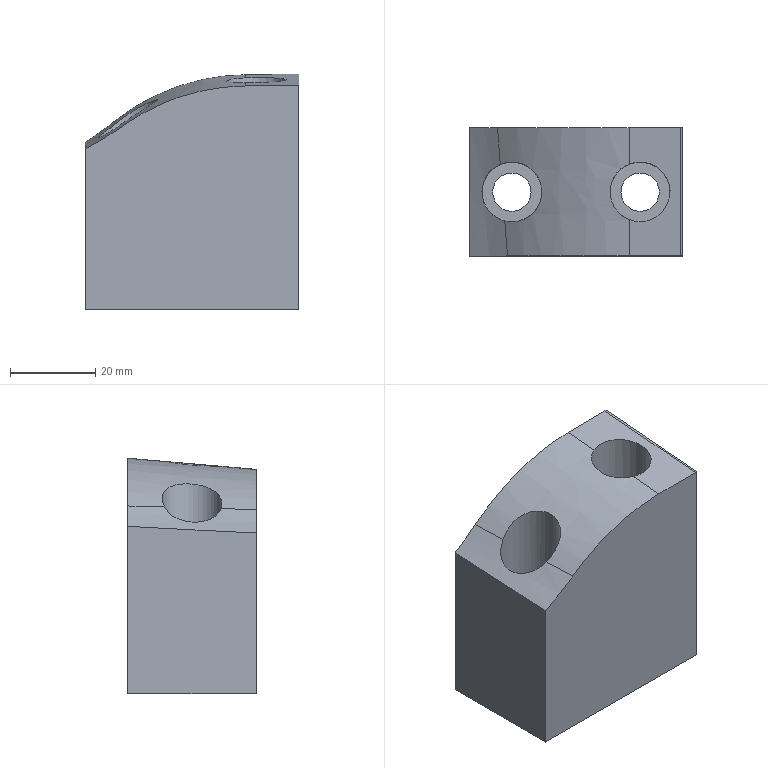Part | NX | features solid 2 | 1 solid | 15 faces | box 50 x 30 x 55.131 mm | volume 61249 mm3 | plane 7 | cylinder 4 | spline 4 | commonest cylinder face diameters 9 x2 14 x2
STEP:
#1=CARTESIAN_POINT('',(822.5,150.,1.131));
#2=VERTEX_POINT('',#1);
#3=CARTESIAN_POINT('',(822.5,150.,-54.));
#4=VERTEX_POINT('',#3);
#5=CARTESIAN_POINT('',(822.5,150.,41.));
#6=DIRECTION('',(0.,0.,-1.));
#7=VECTOR('',#6,1000.);
#8=LINE('',#5,#7);
#9=EDGE_CURVE('',#2,#4,#8,.T.);
#10=ORIENTED_EDGE('',*,*,#9,.F.);
#11=CARTESIAN_POINT('',(822.5,120.,-1.493));
#12=VERTEX_POINT('',#11);
#13=CARTESIAN_POINT('',(822.5,153.462,1.434));
#14=DIRECTION('',(0.,-0.9962,-0.08716));
#15=VECTOR('',#14,1000.);
#16=LINE('',#13,#15);
#17=EDGE_CURVE('',#2,#12,#16,.T.);
#18=ORIENTED_EDGE('',*,*,#17,.T.);
#19=CARTESIAN_POINT('',(822.5,120.,-54.));
#20=VERTEX_POINT('',#19);
#21=CARTESIAN_POINT('',(822.5,120.,41.));
#22=DIRECTION('',(0.,0.,-1.));
#23=VECTOR('',#22,1000.);
#24=LINE('',#21,#23);
#25=EDGE_CURVE('',#12,#20,#24,.T.);
#26=ORIENTED_EDGE('',*,*,#25,.T.);
#27=CARTESIAN_POINT('',(822.5,150.,-54.));
#28=DIRECTION('',(0.,1.,0.));
#29=VECTOR('',#28,1000.);
#30=LINE('',#27,#29);
#31=EDGE_CURVE('',#4,#20,#30,.F.);
#32=ORIENTED_EDGE('',*,*,#31,.F.);
#33=EDGE_LOOP('',(#10,#18,#26,#32));
#34=FACE_BOUND('',#33,.T.);
#35=CARTESIAN_POINT('',(822.5,150.,41.));
#36=DIRECTION('',(1.,0.,0.));
#37=DIRECTION('',(0.,0.,-1.));
#38=AXIS2_PLACEMENT_3D('',#35,#36,#37);
#39=PLANE('',#38);
#40=ADVANCED_FACE('',(#34),#39,.T.);
#41=CARTESIAN_POINT('',(805.5,135.,-44.));
#42=VERTEX_POINT('',#41);
#43=CARTESIAN_POINT('',(812.5,135.,-44.));
#44=DIRECTION('',(0.,0.,-1.));
#45=DIRECTION('',(-1.,0.,0.));
#46=AXIS2_PLACEMENT_3D('',#43,#44,#45);
#47=CIRCLE('',#46,7.);
#48=EDGE_CURVE('',#42,#42,#47,.T.);
#49=ORIENTED_EDGE('',*,*,#48,.T.);
#50=EDGE_LOOP('',(#49));
#51=FACE_BOUND('',#50,.T.);
#52=CARTESIAN_POINT('',(809.928,128.49,-0.8829));
#53=VERTEX_POINT('',#52);
#54=CARTESIAN_POINT('',(809.924,141.509,0.2561));
#55=VERTEX_POINT('',#54);
#56=CARTESIAN_POINT('',(809.929,128.489,-0.8829));
#57=CARTESIAN_POINT('',(808.616,129.008,-0.8514));
#58=CARTESIAN_POINT('',(806.357,130.826,-0.826));
#59=CARTESIAN_POINT('',(805.067,135.021,-0.6039));
#60=CARTESIAN_POINT('',(806.373,139.185,-0.09322));
#61=CARTESIAN_POINT('',(808.613,140.99,0.1969));
#62=CARTESIAN_POINT('',(809.924,141.509,0.2561));
#63=B_SPLINE_CURVE_WITH_KNOTS('',3,(#56,#57,#58,#59,#60,#61,#62),.UNSPECIFIED.,.F.,.F.,(4,1,1,1,4),(0.,0.004174,0.008348,0.01252,0.0167),.UNSPECIFIED.);
#64=EDGE_CURVE('',#53,#55,#63,.T.);
#65=ORIENTED_EDGE('',*,*,#64,.F.);
#66=CARTESIAN_POINT('',(809.923,141.509,0.2561));
#67=CARTESIAN_POINT('',(812.027,142.341,0.351));
#68=CARTESIAN_POINT('',(817.119,141.772,0.3547));
#69=CARTESIAN_POINT('',(820.693,134.994,-0.2007));
#70=CARTESIAN_POINT('',(817.109,128.237,-0.8296));
#71=CARTESIAN_POINT('',(812.055,127.649,-0.9341));
#72=CARTESIAN_POINT('',(809.927,128.49,-0.8829));
#73=B_SPLINE_CURVE_WITH_KNOTS('',3,(#66,#67,#68,#69,#70,#71,#72),.UNSPECIFIED.,.F.,.F.,(4,1,1,1,4),(0.008341,0.01514,0.02193,0.02872,0.03552),.UNSPECIFIED.);
#74=EDGE_CURVE('',#55,#53,#73,.T.);
#75=ORIENTED_EDGE('',*,*,#74,.F.);
#76=EDGE_LOOP('',(#65,#75));
#77=FACE_BOUND('',#76,.T.);
#78=CARTESIAN_POINT('',(812.5,135.,41.));
#79=DIRECTION('',(0.,0.,-1.));
#80=DIRECTION('',(-1.,0.,0.));
#81=AXIS2_PLACEMENT_3D('',#78,#79,#80);
#82=CYLINDRICAL_SURFACE('',#81,7.);
#83=ADVANCED_FACE('',(#51,#77),#82,.F.);
#84=CARTESIAN_POINT('',(775.5,135.,-44.));
#85=VERTEX_POINT('',#84);
#86=CARTESIAN_POINT('',(782.5,135.,-44.));
#87=DIRECTION('',(0.,0.,-1.));
#88=DIRECTION('',(-1.,0.,0.));
#89=AXIS2_PLACEMENT_3D('',#86,#87,#88);
#90=CIRCLE('',#89,7.);
#91=EDGE_CURVE('',#85,#85,#90,.T.);
#92=ORIENTED_EDGE('',*,*,#91,.T.);
#93=EDGE_LOOP('',(#92));
#94=FACE_BOUND('',#93,.T.);
#95=CARTESIAN_POINT('',(779.784,141.451,-10.294));
#96=VERTEX_POINT('',#95);
#97=CARTESIAN_POINT('',(780.817,128.205,-10.671));
#98=VERTEX_POINT('',#97);
#99=CARTESIAN_POINT('',(779.784,141.451,-10.294));
#100=CARTESIAN_POINT('',(780.681,141.829,-9.561));
#101=CARTESIAN_POINT('',(782.626,142.218,-8.111));
#102=CARTESIAN_POINT('',(785.785,141.482,-6.226));
#103=CARTESIAN_POINT('',(788.514,139.168,-5.014));
#104=CARTESIAN_POINT('',(789.811,135.579,-4.738));
#105=CARTESIAN_POINT('',(789.108,131.88,-5.377));
#106=CARTESIAN_POINT('',(786.834,129.171,-6.736));
#107=CARTESIAN_POINT('',(783.84,127.898,-8.579));
#108=CARTESIAN_POINT('',(781.792,127.964,-9.973));
#109=CARTESIAN_POINT('',(780.818,128.205,-10.671));
#110=B_SPLINE_CURVE_WITH_KNOTS('',3,(#99,#100,#101,#102,#103,#104,#105,#106,#107,#108,#109),.UNSPECIFIED.,.F.,.F.,(4,1,1,1,1,1,1,1,4),(0.009346,0.01299,0.01663,0.02027,0.02391,0.02755,0.03119,0.03483,0.03847),.UNSPECIFIED.);
#111=EDGE_CURVE('',#96,#98,#110,.T.);
#112=ORIENTED_EDGE('',*,*,#111,.F.);
#113=CARTESIAN_POINT('',(779.784,141.451,-10.294));
#114=CARTESIAN_POINT('',(778.607,140.956,-11.254));
#115=CARTESIAN_POINT('',(776.389,139.3,-12.978));
#116=CARTESIAN_POINT('',(774.925,134.527,-14.202));
#117=CARTESIAN_POINT('',(776.996,129.903,-13.211));
#118=CARTESIAN_POINT('',(779.54,128.522,-11.587));
#119=CARTESIAN_POINT('',(780.816,128.205,-10.672));
#120=B_SPLINE_CURVE_WITH_KNOTS('',3,(#113,#114,#115,#116,#117,#118,#119),.UNSPECIFIED.,.F.,.F.,(4,1,1,1,4),(0.,0.004707,0.009414,0.01412,0.01883),.UNSPECIFIED.);
#121=EDGE_CURVE('',#96,#98,#120,.T.);
#122=ORIENTED_EDGE('',*,*,#121,.T.);
#123=EDGE_LOOP('',(#112,#122));
#124=FACE_BOUND('',#123,.T.);
#125=CARTESIAN_POINT('',(782.5,135.,41.));
#126=DIRECTION('',(0.,0.,-1.));
#127=DIRECTION('',(-1.,0.,0.));
#128=AXIS2_PLACEMENT_3D('',#125,#126,#127);
#129=CYLINDRICAL_SURFACE('',#128,7.);
#130=ADVANCED_FACE('',(#94,#124),#129,.F.);
#131=CARTESIAN_POINT('',(779.144,150.,-10.05));
#132=VERTEX_POINT('',#131);
#133=CARTESIAN_POINT('',(772.5,150.,-14.808));
#134=VERTEX_POINT('',#133);
#135=CARTESIAN_POINT('',(779.144,150.,-10.05));
#136=CARTESIAN_POINT('',(777.019,150.,-11.762));
#137=CARTESIAN_POINT('',(774.805,150.,-13.348));
#138=CARTESIAN_POINT('',(772.5,150.,-14.808));
#139=B_SPLINE_CURVE_WITH_KNOTS('',3,(#135,#136,#137,#138),.UNSPECIFIED.,.F.,.F.,(4,4),(0.,0.008172),.UNSPECIFIED.);
#140=EDGE_CURVE('',#132,#134,#139,.T.);
#141=ORIENTED_EDGE('',*,*,#140,.F.);
#142=CARTESIAN_POINT('',(809.92,150.,0.9989));
#143=VERTEX_POINT('',#142);
#144=CARTESIAN_POINT('',(779.144,150.,-10.05));
#145=CARTESIAN_POINT('',(781.291,150.,-8.319));
#146=CARTESIAN_POINT('',(785.926,150.,-5.181));
#147=CARTESIAN_POINT('',(796.008,150.,-0.576));
#148=CARTESIAN_POINT('',(804.326,150.,0.9401));
#149=CARTESIAN_POINT('',(809.921,150.,0.9989));
#150=B_SPLINE_CURVE_WITH_KNOTS('',3,(#144,#145,#146,#147,#148,#149),.UNSPECIFIED.,.F.,.F.,(4,1,1,4),(0.009236,0.01751,0.02578,0.04233),.UNSPECIFIED.);
#151=EDGE_CURVE('',#132,#143,#150,.T.);
#152=ORIENTED_EDGE('',*,*,#151,.T.);
#153=CARTESIAN_POINT('',(821.971,150.,1.126));
#154=VERTEX_POINT('',#153);
#155=CARTESIAN_POINT('',(809.92,150.,0.9989));
#156=CARTESIAN_POINT('',(813.937,150.,1.041));
#157=CARTESIAN_POINT('',(817.954,150.,1.083));
#158=CARTESIAN_POINT('',(821.971,150.,1.126));
#159=B_SPLINE_CURVE_WITH_KNOTS('',3,(#155,#156,#157,#158),.UNSPECIFIED.,.F.,.F.,(4,4),(0.007434,0.01949),.UNSPECIFIED.);
#160=EDGE_CURVE('',#143,#154,#159,.T.);
#161=ORIENTED_EDGE('',*,*,#160,.T.);
#162=CARTESIAN_POINT('',(822.919,150.,1.136));
#163=DIRECTION('',(-0.9999,0.,-0.01051));
#164=VECTOR('',#163,1000.);
#165=LINE('',#162,#164);
#166=EDGE_CURVE('',#154,#2,#165,.F.);
#167=ORIENTED_EDGE('',*,*,#166,.T.);
#168=ORIENTED_EDGE('',*,*,#9,.T.);
#169=CARTESIAN_POINT('',(772.5,150.,-54.));
#170=VERTEX_POINT('',#169);
#171=CARTESIAN_POINT('',(822.5,150.,-54.));
#172=DIRECTION('',(-1.,0.,0.));
#173=VECTOR('',#172,1000.);
#174=LINE('',#171,#173);
#175=EDGE_CURVE('',#4,#170,#174,.T.);
#176=ORIENTED_EDGE('',*,*,#175,.T.);
#177=CARTESIAN_POINT('',(772.5,150.,41.));
#178=DIRECTION('',(0.,0.,-1.));
#179=VECTOR('',#178,1000.);
#180=LINE('',#177,#179);
#181=EDGE_CURVE('',#134,#170,#180,.T.);
#182=ORIENTED_EDGE('',*,*,#181,.F.);
#183=EDGE_LOOP('',(#141,#152,#161,#167,#168,#176,#182));
#184=FACE_BOUND('',#183,.T.);
#185=CARTESIAN_POINT('',(822.5,150.,41.));
#186=DIRECTION('',(0.,-1.,0.));
#187=DIRECTION('',(0.,0.,-1.));
#188=AXIS2_PLACEMENT_3D('',#185,#186,#187);
#189=PLANE('',#188);
#190=ADVANCED_FACE('',(#184),#189,.F.);
#191=CARTESIAN_POINT('',(787.,135.,-54.));
#192=VERTEX_POINT('',#191);
#193=CARTESIAN_POINT('',(782.5,135.,-54.));
#194=DIRECTION('',(0.,0.,1.));
#195=DIRECTION('',(1.,0.,0.));
#196=AXIS2_PLACEMENT_3D('',#193,#194,#195);
#197=CIRCLE('',#196,4.5);
#198=EDGE_CURVE('',#192,#192,#197,.F.);
#199=ORIENTED_EDGE('',*,*,#198,.F.);
#200=EDGE_LOOP('',(#199));
#201=FACE_BOUND('',#200,.T.);
#202=CARTESIAN_POINT('',(817.,135.,-54.));
#203=VERTEX_POINT('',#202);
#204=CARTESIAN_POINT('',(812.5,135.,-54.));
#205=DIRECTION('',(0.,0.,1.));
#206=DIRECTION('',(1.,0.,0.));
#207=AXIS2_PLACEMENT_3D('',#204,#205,#206);
#208=CIRCLE('',#207,4.5);
#209=EDGE_CURVE('',#203,#203,#208,.F.);
#210=ORIENTED_EDGE('',*,*,#209,.F.);
#211=EDGE_LOOP('',(#210));
#212=FACE_BOUND('',#211,.T.);
#213=ORIENTED_EDGE('',*,*,#175,.F.);
#214=ORIENTED_EDGE('',*,*,#31,.T.);
#215=CARTESIAN_POINT('',(772.5,120.,-54.));
#216=VERTEX_POINT('',#215);
#217=CARTESIAN_POINT('',(822.5,120.,-54.));
#218=DIRECTION('',(1.,0.,0.));
#219=VECTOR('',#218,1000.);
#220=LINE('',#217,#219);
#221=EDGE_CURVE('',#20,#216,#220,.F.);
#222=ORIENTED_EDGE('',*,*,#221,.T.);
#223=CARTESIAN_POINT('',(772.5,150.,-54.));
#224=DIRECTION('',(0.,1.,0.));
#225=VECTOR('',#224,1000.);
#226=LINE('',#223,#225);
#227=EDGE_CURVE('',#170,#216,#226,.F.);
#228=ORIENTED_EDGE('',*,*,#227,.F.);
#229=EDGE_LOOP('',(#213,#214,#222,#228));
#230=FACE_BOUND('',#229,.T.);
#231=CARTESIAN_POINT('',(822.5,150.,-54.));
#232=DIRECTION('',(0.,0.,1.));
#233=DIRECTION('',(0.,-1.,0.));
#234=AXIS2_PLACEMENT_3D('',#231,#232,#233);
#235=PLANE('',#234);
#236=ADVANCED_FACE('',(#201,#212,#230),#235,.F.);
#237=CARTESIAN_POINT('',(772.5,120.,-16.381));
#238=VERTEX_POINT('',#237);
#239=CARTESIAN_POINT('',(781.483,120.,-10.907));
#240=VERTEX_POINT('',#239);
#241=CARTESIAN_POINT('',(772.5,120.,-16.381));
#242=CARTESIAN_POINT('',(775.626,120.,-14.774));
#243=CARTESIAN_POINT('',(778.62,120.,-12.95));
#244=CARTESIAN_POINT('',(781.481,120.,-10.908));
#245=B_SPLINE_CURVE_WITH_KNOTS('',3,(#241,#242,#243,#244),.UNSPECIFIED.,.F.,.F.,(4,4),(0.,0.01052),.UNSPECIFIED.);
#246=EDGE_CURVE('',#238,#240,#245,.T.);
#247=ORIENTED_EDGE('',*,*,#246,.F.);
#248=CARTESIAN_POINT('',(772.5,120.,41.));
#249=DIRECTION('',(0.,0.,-1.));
#250=VECTOR('',#249,1000.);
#251=LINE('',#248,#250);
#252=EDGE_CURVE('',#238,#216,#251,.T.);
#253=ORIENTED_EDGE('',*,*,#252,.T.);
#254=ORIENTED_EDGE('',*,*,#221,.F.);
#255=ORIENTED_EDGE('',*,*,#25,.F.);
#256=CARTESIAN_POINT('',(821.971,120.,-1.499));
#257=VERTEX_POINT('',#256);
#258=CARTESIAN_POINT('',(822.947,120.,-1.489));
#259=DIRECTION('',(-0.9999,0.,-0.01051));
#260=VECTOR('',#259,1000.);
#261=LINE('',#258,#260);
#262=EDGE_CURVE('',#12,#257,#261,.T.);
#263=ORIENTED_EDGE('',*,*,#262,.T.);
#264=CARTESIAN_POINT('',(809.929,120.,-1.626));
#265=VERTEX_POINT('',#264);
#266=CARTESIAN_POINT('',(821.971,120.,-1.499));
#267=CARTESIAN_POINT('',(817.957,120.,-1.541));
#268=CARTESIAN_POINT('',(813.943,120.,-1.583));
#269=CARTESIAN_POINT('',(809.929,120.,-1.626));
#270=B_SPLINE_CURVE_WITH_KNOTS('',3,(#266,#267,#268,#269),.UNSPECIFIED.,.F.,.F.,(4,4),(0.,0.01204),.UNSPECIFIED.);
#271=EDGE_CURVE('',#257,#265,#270,.T.);
#272=ORIENTED_EDGE('',*,*,#271,.T.);
#273=CARTESIAN_POINT('',(809.93,120.,-1.626));
#274=CARTESIAN_POINT('',(804.815,120.,-1.679));
#275=CARTESIAN_POINT('',(797.323,120.,-2.914));
#276=CARTESIAN_POINT('',(787.852,120.,-6.826));
#277=CARTESIAN_POINT('',(783.548,120.,-9.433));
#278=CARTESIAN_POINT('',(781.484,120.,-10.906));
#279=B_SPLINE_CURVE_WITH_KNOTS('',3,(#273,#274,#275,#276,#277,#278),.UNSPECIFIED.,.F.,.F.,(4,1,1,4),(0.,0.01513,0.0227,0.03026),.UNSPECIFIED.);
#280=EDGE_CURVE('',#265,#240,#279,.T.);
#281=ORIENTED_EDGE('',*,*,#280,.T.);
#282=EDGE_LOOP('',(#247,#253,#254,#255,#263,#272,#281));
#283=FACE_BOUND('',#282,.T.);
#284=CARTESIAN_POINT('',(822.5,120.,41.));
#285=DIRECTION('',(0.,-1.,0.));
#286=DIRECTION('',(0.,0.,-1.));
#287=AXIS2_PLACEMENT_3D('',#284,#285,#286);
#288=PLANE('',#287);
#289=ADVANCED_FACE('',(#283),#288,.T.);
#290=ORIENTED_EDGE('',*,*,#252,.F.);
#291=CARTESIAN_POINT('',(772.5,120.,-16.381));
#292=CARTESIAN_POINT('',(772.5,130.003,-15.905));
#293=CARTESIAN_POINT('',(772.5,140.002,-15.38));
#294=CARTESIAN_POINT('',(772.5,150.,-14.808));
#295=B_SPLINE_CURVE_WITH_KNOTS('',3,(#291,#292,#293,#294),.UNSPECIFIED.,.F.,.F.,(4,4),(0.,0.03004),.UNSPECIFIED.);
#296=EDGE_CURVE('',#238,#134,#295,.T.);
#297=ORIENTED_EDGE('',*,*,#296,.T.);
#298=ORIENTED_EDGE('',*,*,#181,.T.);
#299=ORIENTED_EDGE('',*,*,#227,.T.);
#300=EDGE_LOOP('',(#290,#297,#298,#299));
#301=FACE_BOUND('',#300,.T.);
#302=CARTESIAN_POINT('',(772.5,150.,41.));
#303=DIRECTION('',(1.,0.,0.));
#304=DIRECTION('',(0.,0.,-1.));
#305=AXIS2_PLACEMENT_3D('',#302,#303,#304);
#306=PLANE('',#305);
#307=ADVANCED_FACE('',(#301),#306,.F.);
#308=ORIENTED_EDGE('',*,*,#209,.T.);
#309=EDGE_LOOP('',(#308));
#310=FACE_BOUND('',#309,.T.);
#311=CARTESIAN_POINT('',(808.,135.,-44.));
#312=VERTEX_POINT('',#311);
#313=CARTESIAN_POINT('',(812.5,135.,-44.));
#314=DIRECTION('',(0.,0.,-1.));
#315=DIRECTION('',(-1.,0.,0.));
#316=AXIS2_PLACEMENT_3D('',#313,#314,#315);
#317=CIRCLE('',#316,4.5);
#318=EDGE_CURVE('',#312,#312,#317,.T.);
#319=ORIENTED_EDGE('',*,*,#318,.F.);
#320=EDGE_LOOP('',(#319));
#321=FACE_BOUND('',#320,.T.);
#322=CARTESIAN_POINT('',(812.5,135.,-109.));
#323=DIRECTION('',(0.,0.,-1.));
#324=DIRECTION('',(-1.,0.,0.));
#325=AXIS2_PLACEMENT_3D('',#322,#323,#324);
#326=CYLINDRICAL_SURFACE('',#325,4.5);
#327=ADVANCED_FACE('',(#310,#321),#326,.F.);
#328=ORIENTED_EDGE('',*,*,#318,.T.);
#329=EDGE_LOOP('',(#328));
#330=FACE_BOUND('',#329,.T.);
#331=ORIENTED_EDGE('',*,*,#48,.F.);
#332=EDGE_LOOP('',(#331));
#333=FACE_BOUND('',#332,.T.);
#334=CARTESIAN_POINT('',(812.5,135.,-44.));
#335=DIRECTION('',(0.,0.,-1.));
#336=DIRECTION('',(-1.,0.,0.));
#337=AXIS2_PLACEMENT_3D('',#334,#335,#336);
#338=PLANE('',#337);
#339=ADVANCED_FACE('',(#330,#333),#338,.F.);
#340=ORIENTED_EDGE('',*,*,#198,.T.);
#341=EDGE_LOOP('',(#340));
#342=FACE_BOUND('',#341,.T.);
#343=CARTESIAN_POINT('',(778.,135.,-44.));
#344=VERTEX_POINT('',#343);
#345=CARTESIAN_POINT('',(782.5,135.,-44.));
#346=DIRECTION('',(0.,0.,-1.));
#347=DIRECTION('',(-1.,0.,0.));
#348=AXIS2_PLACEMENT_3D('',#345,#346,#347);
#349=CIRCLE('',#348,4.5);
#350=EDGE_CURVE('',#344,#344,#349,.T.);
#351=ORIENTED_EDGE('',*,*,#350,.F.);
#352=EDGE_LOOP('',(#351));
#353=FACE_BOUND('',#352,.T.);
#354=CARTESIAN_POINT('',(782.5,135.,-109.));
#355=DIRECTION('',(0.,0.,-1.));
#356=DIRECTION('',(-1.,0.,0.));
#357=AXIS2_PLACEMENT_3D('',#354,#355,#356);
#358=CYLINDRICAL_SURFACE('',#357,4.5);
#359=ADVANCED_FACE('',(#342,#353),#358,.F.);
#360=ORIENTED_EDGE('',*,*,#350,.T.);
#361=EDGE_LOOP('',(#360));
#362=FACE_BOUND('',#361,.T.);
#363=ORIENTED_EDGE('',*,*,#91,.F.);
#364=EDGE_LOOP('',(#363));
#365=FACE_BOUND('',#364,.T.);
#366=CARTESIAN_POINT('',(782.5,135.,-44.));
#367=DIRECTION('',(0.,0.,-1.));
#368=DIRECTION('',(-1.,0.,0.));
#369=AXIS2_PLACEMENT_3D('',#366,#367,#368);
#370=PLANE('',#369);
#371=ADVANCED_FACE('',(#362,#365),#370,.F.);
#372=ORIENTED_EDGE('',*,*,#160,.F.);
#373=CARTESIAN_POINT('',(809.923,141.509,0.2561));
#374=CARTESIAN_POINT('',(809.922,144.249,0.4958));
#375=CARTESIAN_POINT('',(809.921,147.08,0.7434));
#376=CARTESIAN_POINT('',(809.92,150.,0.9989));
#377=B_SPLINE_CURVE_WITH_KNOTS('',3,(#373,#374,#375,#376),.UNSPECIFIED.,.F.,.F.,(4,4),(0.8378,0.8517),.UNSPECIFIED.);
#378=EDGE_CURVE('',#55,#143,#377,.T.);
#379=ORIENTED_EDGE('',*,*,#378,.F.);
#380=ORIENTED_EDGE('',*,*,#74,.T.);
#381=CARTESIAN_POINT('',(809.929,120.,-1.626));
#382=CARTESIAN_POINT('',(809.929,122.697,-1.39));
#383=CARTESIAN_POINT('',(809.928,125.527,-1.142));
#384=CARTESIAN_POINT('',(809.927,128.49,-0.8829));
#385=B_SPLINE_CURVE_WITH_KNOTS('',3,(#381,#382,#383,#384),.UNSPECIFIED.,.F.,.F.,(4,4),(0.7976,0.8145),.UNSPECIFIED.);
#386=EDGE_CURVE('',#265,#53,#385,.T.);
#387=ORIENTED_EDGE('',*,*,#386,.F.);
#388=ORIENTED_EDGE('',*,*,#271,.F.);
#389=CARTESIAN_POINT('',(821.971,120.,-1.499));
#390=CARTESIAN_POINT('',(821.971,130.,-0.6242));
#391=CARTESIAN_POINT('',(821.971,140.,0.2507));
#392=CARTESIAN_POINT('',(821.971,150.,1.126));
#393=B_SPLINE_CURVE_WITH_KNOTS('',3,(#389,#390,#391,#392),.UNSPECIFIED.,.F.,.F.,(4,4),(0.3207,0.505),.UNSPECIFIED.);
#394=EDGE_CURVE('',#154,#257,#393,.F.);
#395=ORIENTED_EDGE('',*,*,#394,.F.);
#396=EDGE_LOOP('',(#372,#379,#380,#387,#388,#395));
#397=FACE_BOUND('',#396,.T.);
#398=CARTESIAN_POINT('',(809.848,119.82,-1.642));
#399=CARTESIAN_POINT('',(809.848,150.191,1.015));
#400=CARTESIAN_POINT('',(821.971,119.809,-1.516));
#401=CARTESIAN_POINT('',(821.971,150.18,1.141));
#402=B_SPLINE_SURFACE_WITH_KNOTS('',1,1,((#398,#399),(#400,#401)),.PLANE_SURF.,.F.,.F.,.F.,(2,2),(2,2),(0.8696,1.),(0.8254,0.8716),.PIECEWISE_BEZIER_KNOTS.);
#403=ADVANCED_FACE('',(#397),#402,.T.);
#404=ORIENTED_EDGE('',*,*,#151,.F.);
#405=CARTESIAN_POINT('',(779.144,150.,-10.05));
#406=CARTESIAN_POINT('',(779.249,148.57,-10.091));
#407=CARTESIAN_POINT('',(779.409,146.415,-10.152));
#408=CARTESIAN_POINT('',(779.624,143.552,-10.234));
#409=CARTESIAN_POINT('',(779.735,142.086,-10.276));
#410=CARTESIAN_POINT('',(779.784,141.451,-10.294));
#411=B_SPLINE_CURVE_WITH_KNOTS('',3,(#405,#406,#407,#408,#409,#410),.UNSPECIFIED.,.F.,.F.,(4,1,1,4),(0.2278,0.2397,0.2456,0.2516),.UNSPECIFIED.);
#412=EDGE_CURVE('',#132,#96,#411,.T.);
#413=ORIENTED_EDGE('',*,*,#412,.T.);
#414=ORIENTED_EDGE('',*,*,#111,.T.);
#415=CARTESIAN_POINT('',(780.818,128.205,-10.671));
#416=CARTESIAN_POINT('',(781.035,125.499,-10.748));
#417=CARTESIAN_POINT('',(781.257,122.764,-10.826));
#418=CARTESIAN_POINT('',(781.484,120.,-10.906));
#419=B_SPLINE_CURVE_WITH_KNOTS('',3,(#415,#416,#417,#418),.UNSPECIFIED.,.F.,.F.,(4,4),(0.2921,0.3165),.UNSPECIFIED.);
#420=EDGE_CURVE('',#98,#240,#419,.T.);
#421=ORIENTED_EDGE('',*,*,#420,.T.);
#422=ORIENTED_EDGE('',*,*,#280,.F.);
#423=ORIENTED_EDGE('',*,*,#386,.T.);
#424=ORIENTED_EDGE('',*,*,#64,.T.);
#425=ORIENTED_EDGE('',*,*,#378,.T.);
#426=EDGE_LOOP('',(#404,#413,#414,#421,#422,#423,#424,#425));
#427=FACE_BOUND('',#426,.T.);
#428=CARTESIAN_POINT('',(809.93,119.012,-1.712));
#429=CARTESIAN_POINT('',(792.527,119.027,-1.894));
#430=CARTESIAN_POINT('',(778.998,119.979,-12.802));
#431=CARTESIAN_POINT('',(809.929,129.403,-0.803));
#432=CARTESIAN_POINT('',(792.526,129.414,-0.985));
#433=CARTESIAN_POINT('',(778.997,130.364,-11.893));
#434=CARTESIAN_POINT('',(809.925,139.794,0.1061));
#435=CARTESIAN_POINT('',(792.522,139.803,-0.07612));
#436=CARTESIAN_POINT('',(778.993,140.751,-10.984));
#437=CARTESIAN_POINT('',(809.921,150.185,1.015));
#438=CARTESIAN_POINT('',(792.517,150.193,0.8329));
#439=CARTESIAN_POINT('',(778.988,151.141,-10.076));
#440=(BOUNDED_SURFACE()B_SPLINE_SURFACE(3,2,((#428,#429,#430),(#431,#432,#433),(#434,#435,#436),(#437,#438,#439)),.UNSPECIFIED.,.F.,.F.,.F.)B_SPLINE_SURFACE_WITH_KNOTS((4,4),(3,3),(0.5972,0.6285),(0.,0.7758),.PIECEWISE_BEZIER_KNOTS.)GEOMETRIC_REPRESENTATION_ITEM()RATIONAL_B_SPLINE_SURFACE(((1.,0.9293,0.9683),(1.,0.9293,0.9683),(1.,0.9293,0.9683),(1.,0.9293,0.9683)))REPRESENTATION_ITEM('')SURFACE());
#441=ADVANCED_FACE('',(#427),#440,.T.);
#442=ORIENTED_EDGE('',*,*,#412,.F.);
#443=ORIENTED_EDGE('',*,*,#140,.T.);
#444=ORIENTED_EDGE('',*,*,#296,.F.);
#445=ORIENTED_EDGE('',*,*,#246,.T.);
#446=ORIENTED_EDGE('',*,*,#420,.F.);
#447=ORIENTED_EDGE('',*,*,#121,.F.);
#448=EDGE_LOOP('',(#442,#443,#444,#445,#446,#447));
#449=FACE_BOUND('',#448,.T.);
#450=CARTESIAN_POINT('',(779.028,151.58,-10.005));
#451=CARTESIAN_POINT('',(774.602,150.617,-13.678));
#452=CARTESIAN_POINT('',(769.632,149.601,-16.552));
#453=CARTESIAN_POINT('',(779.804,140.973,-10.308));
#454=CARTESIAN_POINT('',(775.438,140.004,-13.787));
#455=CARTESIAN_POINT('',(770.571,138.981,-16.504));
#456=CARTESIAN_POINT('',(780.628,130.384,-10.607));
#457=CARTESIAN_POINT('',(776.333,129.409,-13.891));
#458=CARTESIAN_POINT('',(771.582,128.381,-16.45));
#459=CARTESIAN_POINT('',(781.496,119.812,-10.914));
#460=CARTESIAN_POINT('',(777.287,118.827,-14.002));
#461=CARTESIAN_POINT('',(772.661,117.796,-16.403));
#462=(BOUNDED_SURFACE()B_SPLINE_SURFACE(3,2,((#450,#451,#452),(#453,#454,#455),(#456,#457,#458),(#459,#460,#461)),.UNSPECIFIED.,.F.,.F.,.F.)B_SPLINE_SURFACE_WITH_KNOTS((4,4),(3,3),(0.233,0.2655),(0.,0.2396),.PIECEWISE_BEZIER_KNOTS.)GEOMETRIC_REPRESENTATION_ITEM()RATIONAL_B_SPLINE_SURFACE(((1.,0.9855,0.9779),(1.,0.9863,0.9792),(1.,0.9871,0.9805),(1.,0.988,0.9817)))REPRESENTATION_ITEM('')SURFACE());
#463=ADVANCED_FACE('',(#449),#462,.F.);
#464=ORIENTED_EDGE('',*,*,#166,.F.);
#465=ORIENTED_EDGE('',*,*,#394,.T.);
#466=ORIENTED_EDGE('',*,*,#262,.F.);
#467=ORIENTED_EDGE('',*,*,#17,.F.);
#468=EDGE_LOOP('',(#464,#465,#466,#467));
#469=FACE_BOUND('',#468,.T.);
#470=CARTESIAN_POINT('',(821.971,119.82,-1.515));
#471=CARTESIAN_POINT('',(821.971,150.18,1.141));
#472=CARTESIAN_POINT('',(822.5,119.82,-1.509));
#473=CARTESIAN_POINT('',(822.5,150.18,1.147));
#474=B_SPLINE_SURFACE_WITH_KNOTS('',1,1,((#470,#471),(#472,#473)),.PLANE_SURF.,.F.,.F.,.F.,(2,2),(2,2),(0.8699,0.8748),(0.8288,0.8741),.PIECEWISE_BEZIER_KNOTS.);
#475=ADVANCED_FACE('',(#469),#474,.T.);
#476=CLOSED_SHELL('',(#40,#83,#130,#190,#236,#289,#307,#327,#339,#359,#371,#403,#441,#463,#475));
#477=MANIFOLD_SOLID_BREP('',#476);
#478=(LENGTH_UNIT()NAMED_UNIT(*)SI_UNIT(.MILLI.,.METRE.));
#479=UNCERTAINTY_MEASURE_WITH_UNIT(LENGTH_MEASURE(0.05674),#478,'','');
#480=(NAMED_UNIT(*)PLANE_ANGLE_UNIT()SI_UNIT($,.RADIAN.));
#481=(NAMED_UNIT(*)SI_UNIT($,.STERADIAN.)SOLID_ANGLE_UNIT());
#482=(GEOMETRIC_REPRESENTATION_CONTEXT(3)GLOBAL_UNCERTAINTY_ASSIGNED_CONTEXT((#479))GLOBAL_UNIT_ASSIGNED_CONTEXT((#478,#480,#481))REPRESENTATION_CONTEXT('',''));
#483=ADVANCED_BREP_SHAPE_REPRESENTATION('',(#477),#482);